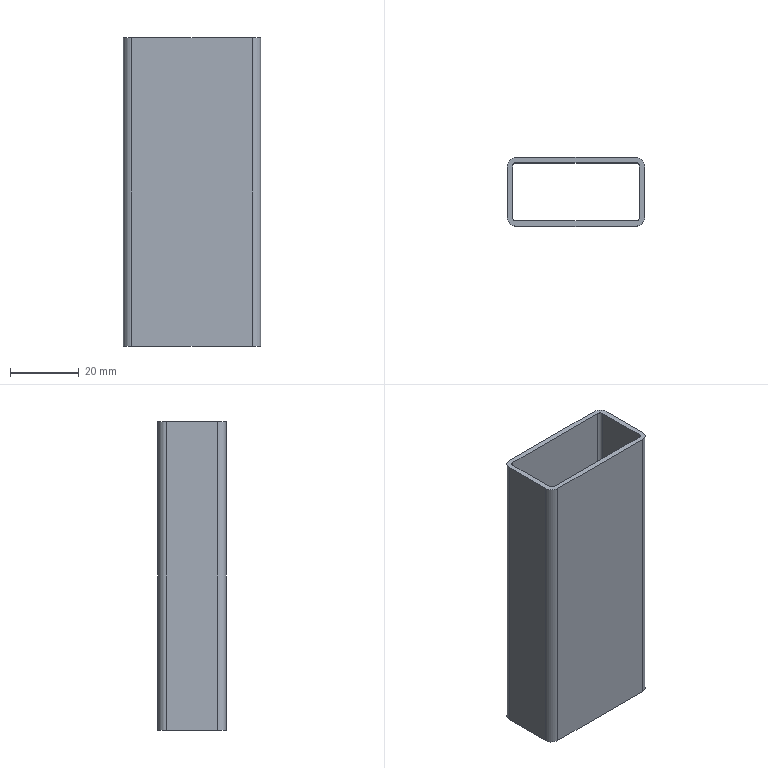Part | STEP file | 6100517 | 1 solid | 18 faces | box 40 x 20 x 90 mm | volume 14984 mm3 | plane 10 | cylinder 8 | commonest cylinder face diameters 2 x4 5 x4
STEP:
#1=CARTESIAN_POINT('',(0.,0.,0.));
#2=DIRECTION('',(0.,0.,1.));
#3=DIRECTION('',(1.,0.,0.));
#4=AXIS2_PLACEMENT_3D('',#1,#2,#3);
#5=CARTESIAN_POINT('',(-17.5,10.,90.));
#6=VERTEX_POINT('',#5);
#7=CARTESIAN_POINT('',(-20.,7.5,90.));
#8=VERTEX_POINT('',#7);
#9=CARTESIAN_POINT('',(-17.5,7.5,90.));
#10=DIRECTION('',(0.,0.,1.));
#11=DIRECTION('',(1.,0.,0.));
#12=AXIS2_PLACEMENT_3D('',#9,#10,#11);
#13=CIRCLE('',#12,2.5);
#14=CARTESIAN_POINT('',(-17.5,7.5,90.));
#15=DIRECTION('',(0.,0.,1.));
#16=DIRECTION('',(1.,0.,0.));
#17=AXIS2_PLACEMENT_3D('',#14,#15,#16);
#18=PLANE('',#17);
#19=CARTESIAN_POINT('',(0.,0.));
#20=DIRECTION('',(1.,0.));
#21=AXIS2_PLACEMENT_2D('',#19,#20);
#22=CIRCLE('',#21,2.5);
#23=(GEOMETRIC_REPRESENTATION_CONTEXT(2)PARAMETRIC_REPRESENTATION_CONTEXT()REPRESENTATION_CONTEXT('',''));
#24=DEFINITIONAL_REPRESENTATION('',(#22),#23);
#25=PCURVE('',#18,#24);
#26=CARTESIAN_POINT('',(-17.5,7.5,90.));
#27=DIRECTION('',(0.,0.,-1.));
#28=DIRECTION('',(-1.,0.,0.));
#29=AXIS2_PLACEMENT_3D('',#26,#27,#28);
#30=CYLINDRICAL_SURFACE('',#29,2.5);
#31=CARTESIAN_POINT('',(3.142,0.));
#32=DIRECTION('',(-1.,0.));
#33=VECTOR('',#32,1.);
#34=LINE('',#31,#33);
#35=(GEOMETRIC_REPRESENTATION_CONTEXT(2)PARAMETRIC_REPRESENTATION_CONTEXT()REPRESENTATION_CONTEXT('',''));
#36=DEFINITIONAL_REPRESENTATION('',(#34),#35);
#37=PCURVE('',#30,#36);
#38=SURFACE_CURVE('',#13,(#25,#37),.PCURVE_S1.);
#39=EDGE_CURVE('',#6,#8,#38,.T.);
#40=ORIENTED_EDGE('',*,*,#39,.T.);
#41=CARTESIAN_POINT('',(-20.,-7.5,90.));
#42=VERTEX_POINT('',#41);
#43=CARTESIAN_POINT('',(-20.,7.5,90.));
#44=DIRECTION('',(0.,-1.,0.));
#45=VECTOR('',#44,1.);
#46=LINE('',#43,#45);
#47=CARTESIAN_POINT('',(-2.5,0.));
#48=DIRECTION('',(0.,-1.));
#49=VECTOR('',#48,1.);
#50=LINE('',#47,#49);
#51=(GEOMETRIC_REPRESENTATION_CONTEXT(2)PARAMETRIC_REPRESENTATION_CONTEXT()REPRESENTATION_CONTEXT('',''));
#52=DEFINITIONAL_REPRESENTATION('',(#50),#51);
#53=PCURVE('',#18,#52);
#54=CARTESIAN_POINT('',(-20.,7.5,90.));
#55=DIRECTION('',(1.,0.,0.));
#56=DIRECTION('',(0.,1.,0.));
#57=AXIS2_PLACEMENT_3D('',#54,#55,#56);
#58=PLANE('',#57);
#59=CARTESIAN_POINT('',(0.,0.));
#60=DIRECTION('',(-1.,0.));
#61=VECTOR('',#60,1.);
#62=LINE('',#59,#61);
#63=(GEOMETRIC_REPRESENTATION_CONTEXT(2)PARAMETRIC_REPRESENTATION_CONTEXT()REPRESENTATION_CONTEXT('',''));
#64=DEFINITIONAL_REPRESENTATION('',(#62),#63);
#65=PCURVE('',#58,#64);
#66=SURFACE_CURVE('',#46,(#53,#65),.PCURVE_S1.);
#67=EDGE_CURVE('',#8,#42,#66,.T.);
#68=ORIENTED_EDGE('',*,*,#67,.T.);
#69=CARTESIAN_POINT('',(-17.5,-10.,90.));
#70=VERTEX_POINT('',#69);
#71=CARTESIAN_POINT('',(-17.5,-7.5,90.));
#72=DIRECTION('',(0.,0.,1.));
#73=DIRECTION('',(1.,0.,0.));
#74=AXIS2_PLACEMENT_3D('',#71,#72,#73);
#75=CIRCLE('',#74,2.5);
#76=CARTESIAN_POINT('',(0.,-15.));
#77=DIRECTION('',(1.,0.));
#78=AXIS2_PLACEMENT_2D('',#76,#77);
#79=CIRCLE('',#78,2.5);
#80=(GEOMETRIC_REPRESENTATION_CONTEXT(2)PARAMETRIC_REPRESENTATION_CONTEXT()REPRESENTATION_CONTEXT('',''));
#81=DEFINITIONAL_REPRESENTATION('',(#79),#80);
#82=PCURVE('',#18,#81);
#83=CARTESIAN_POINT('',(-17.5,-7.5,90.));
#84=DIRECTION('',(0.,0.,-1.));
#85=DIRECTION('',(-1.,0.,0.));
#86=AXIS2_PLACEMENT_3D('',#83,#84,#85);
#87=CYLINDRICAL_SURFACE('',#86,2.5);
#88=CARTESIAN_POINT('',(9.425,0.));
#89=DIRECTION('',(-1.,0.));
#90=VECTOR('',#89,1.);
#91=LINE('',#88,#90);
#92=(GEOMETRIC_REPRESENTATION_CONTEXT(2)PARAMETRIC_REPRESENTATION_CONTEXT()REPRESENTATION_CONTEXT('',''));
#93=DEFINITIONAL_REPRESENTATION('',(#91),#92);
#94=PCURVE('',#87,#93);
#95=SURFACE_CURVE('',#75,(#82,#94),.PCURVE_S1.);
#96=EDGE_CURVE('',#42,#70,#95,.T.);
#97=ORIENTED_EDGE('',*,*,#96,.T.);
#98=CARTESIAN_POINT('',(17.5,-10.,90.));
#99=VERTEX_POINT('',#98);
#100=CARTESIAN_POINT('',(-17.5,-10.,90.));
#101=DIRECTION('',(1.,0.,0.));
#102=VECTOR('',#101,1.);
#103=LINE('',#100,#102);
#104=CARTESIAN_POINT('',(0.,-17.5));
#105=DIRECTION('',(1.,0.));
#106=VECTOR('',#105,1.);
#107=LINE('',#104,#106);
#108=(GEOMETRIC_REPRESENTATION_CONTEXT(2)PARAMETRIC_REPRESENTATION_CONTEXT()REPRESENTATION_CONTEXT('',''));
#109=DEFINITIONAL_REPRESENTATION('',(#107),#108);
#110=PCURVE('',#18,#109);
#111=CARTESIAN_POINT('',(-17.5,-10.,90.));
#112=DIRECTION('',(0.,1.,0.));
#113=DIRECTION('',(0.,0.,1.));
#114=AXIS2_PLACEMENT_3D('',#111,#112,#113);
#115=PLANE('',#114);
#116=CARTESIAN_POINT('',(0.,0.));
#117=DIRECTION('',(0.,1.));
#118=VECTOR('',#117,1.);
#119=LINE('',#116,#118);
#120=(GEOMETRIC_REPRESENTATION_CONTEXT(2)PARAMETRIC_REPRESENTATION_CONTEXT()REPRESENTATION_CONTEXT('',''));
#121=DEFINITIONAL_REPRESENTATION('',(#119),#120);
#122=PCURVE('',#115,#121);
#123=SURFACE_CURVE('',#103,(#110,#122),.PCURVE_S1.);
#124=EDGE_CURVE('',#70,#99,#123,.T.);
#125=ORIENTED_EDGE('',*,*,#124,.T.);
#126=CARTESIAN_POINT('',(20.,-7.5,90.));
#127=VERTEX_POINT('',#126);
#128=CARTESIAN_POINT('',(17.5,-7.5,90.));
#129=DIRECTION('',(0.,0.,1.));
#130=DIRECTION('',(1.,0.,0.));
#131=AXIS2_PLACEMENT_3D('',#128,#129,#130);
#132=CIRCLE('',#131,2.5);
#133=CARTESIAN_POINT('',(35.,-15.));
#134=DIRECTION('',(1.,0.));
#135=AXIS2_PLACEMENT_2D('',#133,#134);
#136=CIRCLE('',#135,2.5);
#137=(GEOMETRIC_REPRESENTATION_CONTEXT(2)PARAMETRIC_REPRESENTATION_CONTEXT()REPRESENTATION_CONTEXT('',''));
#138=DEFINITIONAL_REPRESENTATION('',(#136),#137);
#139=PCURVE('',#18,#138);
#140=CARTESIAN_POINT('',(17.5,-7.5,90.));
#141=DIRECTION('',(0.,0.,-1.));
#142=DIRECTION('',(-1.,0.,0.));
#143=AXIS2_PLACEMENT_3D('',#140,#141,#142);
#144=CYLINDRICAL_SURFACE('',#143,2.5);
#145=CARTESIAN_POINT('',(9.425,0.));
#146=DIRECTION('',(-1.,0.));
#147=VECTOR('',#146,1.);
#148=LINE('',#145,#147);
#149=(GEOMETRIC_REPRESENTATION_CONTEXT(2)PARAMETRIC_REPRESENTATION_CONTEXT()REPRESENTATION_CONTEXT('',''));
#150=DEFINITIONAL_REPRESENTATION('',(#148),#149);
#151=PCURVE('',#144,#150);
#152=SURFACE_CURVE('',#132,(#139,#151),.PCURVE_S1.);
#153=EDGE_CURVE('',#99,#127,#152,.T.);
#154=ORIENTED_EDGE('',*,*,#153,.T.);
#155=CARTESIAN_POINT('',(20.,7.5,90.));
#156=VERTEX_POINT('',#155);
#157=CARTESIAN_POINT('',(20.,7.5,90.));
#158=DIRECTION('',(0.,1.,0.));
#159=VECTOR('',#158,1.);
#160=LINE('',#157,#159);
#161=CARTESIAN_POINT('',(37.5,0.));
#162=DIRECTION('',(0.,1.));
#163=VECTOR('',#162,1.);
#164=LINE('',#161,#163);
#165=(GEOMETRIC_REPRESENTATION_CONTEXT(2)PARAMETRIC_REPRESENTATION_CONTEXT()REPRESENTATION_CONTEXT('',''));
#166=DEFINITIONAL_REPRESENTATION('',(#164),#165);
#167=PCURVE('',#18,#166);
#168=CARTESIAN_POINT('',(20.,7.5,90.));
#169=DIRECTION('',(-1.,0.,0.));
#170=DIRECTION('',(0.,-1.,0.));
#171=AXIS2_PLACEMENT_3D('',#168,#169,#170);
#172=PLANE('',#171);
#173=CARTESIAN_POINT('',(0.,0.));
#174=DIRECTION('',(-1.,0.));
#175=VECTOR('',#174,1.);
#176=LINE('',#173,#175);
#177=(GEOMETRIC_REPRESENTATION_CONTEXT(2)PARAMETRIC_REPRESENTATION_CONTEXT()REPRESENTATION_CONTEXT('',''));
#178=DEFINITIONAL_REPRESENTATION('',(#176),#177);
#179=PCURVE('',#172,#178);
#180=SURFACE_CURVE('',#160,(#167,#179),.PCURVE_S1.);
#181=EDGE_CURVE('',#127,#156,#180,.T.);
#182=ORIENTED_EDGE('',*,*,#181,.T.);
#183=CARTESIAN_POINT('',(17.5,10.,90.));
#184=VERTEX_POINT('',#183);
#185=CARTESIAN_POINT('',(17.5,7.5,90.));
#186=DIRECTION('',(0.,0.,1.));
#187=DIRECTION('',(-1.,0.,0.));
#188=AXIS2_PLACEMENT_3D('',#185,#186,#187);
#189=CIRCLE('',#188,2.5);
#190=CARTESIAN_POINT('',(35.,0.));
#191=DIRECTION('',(-1.,0.));
#192=AXIS2_PLACEMENT_2D('',#190,#191);
#193=CIRCLE('',#192,2.5);
#194=(GEOMETRIC_REPRESENTATION_CONTEXT(2)PARAMETRIC_REPRESENTATION_CONTEXT()REPRESENTATION_CONTEXT('',''));
#195=DEFINITIONAL_REPRESENTATION('',(#193),#194);
#196=PCURVE('',#18,#195);
#197=CARTESIAN_POINT('',(17.5,7.5,90.));
#198=DIRECTION('',(0.,0.,-1.));
#199=DIRECTION('',(-1.,0.,0.));
#200=AXIS2_PLACEMENT_3D('',#197,#198,#199);
#201=CYLINDRICAL_SURFACE('',#200,2.5);
#202=CARTESIAN_POINT('',(6.283,0.));
#203=DIRECTION('',(-1.,0.));
#204=VECTOR('',#203,1.);
#205=LINE('',#202,#204);
#206=(GEOMETRIC_REPRESENTATION_CONTEXT(2)PARAMETRIC_REPRESENTATION_CONTEXT()REPRESENTATION_CONTEXT('',''));
#207=DEFINITIONAL_REPRESENTATION('',(#205),#206);
#208=PCURVE('',#201,#207);
#209=SURFACE_CURVE('',#189,(#196,#208),.PCURVE_S1.);
#210=EDGE_CURVE('',#156,#184,#209,.T.);
#211=ORIENTED_EDGE('',*,*,#210,.T.);
#212=CARTESIAN_POINT('',(-17.5,10.,90.));
#213=DIRECTION('',(-1.,0.,0.));
#214=VECTOR('',#213,1.);
#215=LINE('',#212,#214);
#216=CARTESIAN_POINT('',(0.,2.5));
#217=DIRECTION('',(-1.,0.));
#218=VECTOR('',#217,1.);
#219=LINE('',#216,#218);
#220=(GEOMETRIC_REPRESENTATION_CONTEXT(2)PARAMETRIC_REPRESENTATION_CONTEXT()REPRESENTATION_CONTEXT('',''));
#221=DEFINITIONAL_REPRESENTATION('',(#219),#220);
#222=PCURVE('',#18,#221);
#223=CARTESIAN_POINT('',(-17.5,10.,90.));
#224=DIRECTION('',(0.,-1.,0.));
#225=DIRECTION('',(0.,0.,-1.));
#226=AXIS2_PLACEMENT_3D('',#223,#224,#225);
#227=PLANE('',#226);
#228=CARTESIAN_POINT('',(0.,0.));
#229=DIRECTION('',(0.,-1.));
#230=VECTOR('',#229,1.);
#231=LINE('',#228,#230);
#232=(GEOMETRIC_REPRESENTATION_CONTEXT(2)PARAMETRIC_REPRESENTATION_CONTEXT()REPRESENTATION_CONTEXT('',''));
#233=DEFINITIONAL_REPRESENTATION('',(#231),#232);
#234=PCURVE('',#227,#233);
#235=SURFACE_CURVE('',#215,(#222,#234),.PCURVE_S1.);
#236=EDGE_CURVE('',#184,#6,#235,.T.);
#237=ORIENTED_EDGE('',*,*,#236,.T.);
#238=EDGE_LOOP('',(#40,#68,#97,#125,#154,#182,#211,#237));
#239=FACE_BOUND('',#238,.T.);
#240=CARTESIAN_POINT('',(-18.5,7.5,90.));
#241=VERTEX_POINT('',#240);
#242=CARTESIAN_POINT('',(-18.5,-7.5,90.));
#243=VERTEX_POINT('',#242);
#244=CARTESIAN_POINT('',(-18.5,7.5,90.));
#245=DIRECTION('',(0.,-1.,0.));
#246=VECTOR('',#245,1.);
#247=LINE('',#244,#246);
#248=CARTESIAN_POINT('',(-1.,0.));
#249=DIRECTION('',(0.,-1.));
#250=VECTOR('',#249,1.);
#251=LINE('',#248,#250);
#252=(GEOMETRIC_REPRESENTATION_CONTEXT(2)PARAMETRIC_REPRESENTATION_CONTEXT()REPRESENTATION_CONTEXT('',''));
#253=DEFINITIONAL_REPRESENTATION('',(#251),#252);
#254=PCURVE('',#18,#253);
#255=CARTESIAN_POINT('',(-18.5,7.5,90.));
#256=DIRECTION('',(1.,0.,0.));
#257=DIRECTION('',(0.,0.,-1.));
#258=AXIS2_PLACEMENT_3D('',#255,#256,#257);
#259=PLANE('',#258);
#260=CARTESIAN_POINT('',(0.,0.));
#261=DIRECTION('',(0.,-1.));
#262=VECTOR('',#261,1.);
#263=LINE('',#260,#262);
#264=(GEOMETRIC_REPRESENTATION_CONTEXT(2)PARAMETRIC_REPRESENTATION_CONTEXT()REPRESENTATION_CONTEXT('',''));
#265=DEFINITIONAL_REPRESENTATION('',(#263),#264);
#266=PCURVE('',#259,#265);
#267=SURFACE_CURVE('',#247,(#254,#266),.PCURVE_S1.);
#268=EDGE_CURVE('',#241,#243,#267,.T.);
#269=ORIENTED_EDGE('',*,*,#268,.F.);
#270=CARTESIAN_POINT('',(-17.5,8.5,90.));
#271=VERTEX_POINT('',#270);
#272=CARTESIAN_POINT('',(-17.5,7.5,90.));
#273=DIRECTION('',(0.,0.,1.));
#274=DIRECTION('',(1.,0.,0.));
#275=AXIS2_PLACEMENT_3D('',#272,#273,#274);
#276=CIRCLE('',#275,1.);
#277=CARTESIAN_POINT('',(0.,0.));
#278=DIRECTION('',(1.,0.));
#279=AXIS2_PLACEMENT_2D('',#277,#278);
#280=CIRCLE('',#279,1.);
#281=(GEOMETRIC_REPRESENTATION_CONTEXT(2)PARAMETRIC_REPRESENTATION_CONTEXT()REPRESENTATION_CONTEXT('',''));
#282=DEFINITIONAL_REPRESENTATION('',(#280),#281);
#283=PCURVE('',#18,#282);
#284=CARTESIAN_POINT('',(-17.5,7.5,90.));
#285=DIRECTION('',(0.,0.,-1.));
#286=DIRECTION('',(-1.,0.,0.));
#287=AXIS2_PLACEMENT_3D('',#284,#285,#286);
#288=CYLINDRICAL_SURFACE('',#287,1.);
#289=CARTESIAN_POINT('',(3.142,0.));
#290=DIRECTION('',(-1.,0.));
#291=VECTOR('',#290,1.);
#292=LINE('',#289,#291);
#293=(GEOMETRIC_REPRESENTATION_CONTEXT(2)PARAMETRIC_REPRESENTATION_CONTEXT()REPRESENTATION_CONTEXT('',''));
#294=DEFINITIONAL_REPRESENTATION('',(#292),#293);
#295=PCURVE('',#288,#294);
#296=SURFACE_CURVE('',#276,(#283,#295),.PCURVE_S1.);
#297=EDGE_CURVE('',#271,#241,#296,.T.);
#298=ORIENTED_EDGE('',*,*,#297,.F.);
#299=CARTESIAN_POINT('',(17.5,8.5,90.));
#300=VERTEX_POINT('',#299);
#301=CARTESIAN_POINT('',(-17.5,8.5,90.));
#302=DIRECTION('',(-1.,0.,0.));
#303=VECTOR('',#302,1.);
#304=LINE('',#301,#303);
#305=CARTESIAN_POINT('',(0.,1.));
#306=DIRECTION('',(-1.,0.));
#307=VECTOR('',#306,1.);
#308=LINE('',#305,#307);
#309=(GEOMETRIC_REPRESENTATION_CONTEXT(2)PARAMETRIC_REPRESENTATION_CONTEXT()REPRESENTATION_CONTEXT('',''));
#310=DEFINITIONAL_REPRESENTATION('',(#308),#309);
#311=PCURVE('',#18,#310);
#312=CARTESIAN_POINT('',(-17.5,8.5,90.));
#313=DIRECTION('',(0.,-1.,0.));
#314=DIRECTION('',(0.,0.,-1.));
#315=AXIS2_PLACEMENT_3D('',#312,#313,#314);
#316=PLANE('',#315);
#317=CARTESIAN_POINT('',(0.,0.));
#318=DIRECTION('',(0.,-1.));
#319=VECTOR('',#318,1.);
#320=LINE('',#317,#319);
#321=(GEOMETRIC_REPRESENTATION_CONTEXT(2)PARAMETRIC_REPRESENTATION_CONTEXT()REPRESENTATION_CONTEXT('',''));
#322=DEFINITIONAL_REPRESENTATION('',(#320),#321);
#323=PCURVE('',#316,#322);
#324=SURFACE_CURVE('',#304,(#311,#323),.PCURVE_S1.);
#325=EDGE_CURVE('',#300,#271,#324,.T.);
#326=ORIENTED_EDGE('',*,*,#325,.F.);
#327=CARTESIAN_POINT('',(18.5,7.5,90.));
#328=VERTEX_POINT('',#327);
#329=CARTESIAN_POINT('',(17.5,7.5,90.));
#330=DIRECTION('',(0.,0.,1.));
#331=DIRECTION('',(-1.,0.,0.));
#332=AXIS2_PLACEMENT_3D('',#329,#330,#331);
#333=CIRCLE('',#332,1.);
#334=CARTESIAN_POINT('',(35.,0.));
#335=DIRECTION('',(-1.,0.));
#336=AXIS2_PLACEMENT_2D('',#334,#335);
#337=CIRCLE('',#336,1.);
#338=(GEOMETRIC_REPRESENTATION_CONTEXT(2)PARAMETRIC_REPRESENTATION_CONTEXT()REPRESENTATION_CONTEXT('',''));
#339=DEFINITIONAL_REPRESENTATION('',(#337),#338);
#340=PCURVE('',#18,#339);
#341=CARTESIAN_POINT('',(17.5,7.5,90.));
#342=DIRECTION('',(0.,0.,-1.));
#343=DIRECTION('',(-1.,0.,0.));
#344=AXIS2_PLACEMENT_3D('',#341,#342,#343);
#345=CYLINDRICAL_SURFACE('',#344,1.);
#346=CARTESIAN_POINT('',(6.283,0.));
#347=DIRECTION('',(-1.,0.));
#348=VECTOR('',#347,1.);
#349=LINE('',#346,#348);
#350=(GEOMETRIC_REPRESENTATION_CONTEXT(2)PARAMETRIC_REPRESENTATION_CONTEXT()REPRESENTATION_CONTEXT('',''));
#351=DEFINITIONAL_REPRESENTATION('',(#349),#350);
#352=PCURVE('',#345,#351);
#353=SURFACE_CURVE('',#333,(#340,#352),.PCURVE_S1.);
#354=EDGE_CURVE('',#328,#300,#353,.T.);
#355=ORIENTED_EDGE('',*,*,#354,.F.);
#356=CARTESIAN_POINT('',(18.5,-7.5,90.));
#357=VERTEX_POINT('',#356);
#358=CARTESIAN_POINT('',(18.5,7.5,90.));
#359=DIRECTION('',(0.,1.,0.));
#360=VECTOR('',#359,1.);
#361=LINE('',#358,#360);
#362=CARTESIAN_POINT('',(36.,0.));
#363=DIRECTION('',(0.,1.));
#364=VECTOR('',#363,1.);
#365=LINE('',#362,#364);
#366=(GEOMETRIC_REPRESENTATION_CONTEXT(2)PARAMETRIC_REPRESENTATION_CONTEXT()REPRESENTATION_CONTEXT('',''));
#367=DEFINITIONAL_REPRESENTATION('',(#365),#366);
#368=PCURVE('',#18,#367);
#369=CARTESIAN_POINT('',(18.5,7.5,90.));
#370=DIRECTION('',(-1.,0.,0.));
#371=DIRECTION('',(0.,-1.,0.));
#372=AXIS2_PLACEMENT_3D('',#369,#370,#371);
#373=PLANE('',#372);
#374=CARTESIAN_POINT('',(0.,0.));
#375=DIRECTION('',(-1.,0.));
#376=VECTOR('',#375,1.);
#377=LINE('',#374,#376);
#378=(GEOMETRIC_REPRESENTATION_CONTEXT(2)PARAMETRIC_REPRESENTATION_CONTEXT()REPRESENTATION_CONTEXT('',''));
#379=DEFINITIONAL_REPRESENTATION('',(#377),#378);
#380=PCURVE('',#373,#379);
#381=SURFACE_CURVE('',#361,(#368,#380),.PCURVE_S1.);
#382=EDGE_CURVE('',#357,#328,#381,.T.);
#383=ORIENTED_EDGE('',*,*,#382,.F.);
#384=CARTESIAN_POINT('',(17.5,-8.5,90.));
#385=VERTEX_POINT('',#384);
#386=CARTESIAN_POINT('',(17.5,-7.5,90.));
#387=DIRECTION('',(0.,0.,1.));
#388=DIRECTION('',(1.,0.,0.));
#389=AXIS2_PLACEMENT_3D('',#386,#387,#388);
#390=CIRCLE('',#389,1.);
#391=CARTESIAN_POINT('',(35.,-15.));
#392=DIRECTION('',(1.,0.));
#393=AXIS2_PLACEMENT_2D('',#391,#392);
#394=CIRCLE('',#393,1.);
#395=(GEOMETRIC_REPRESENTATION_CONTEXT(2)PARAMETRIC_REPRESENTATION_CONTEXT()REPRESENTATION_CONTEXT('',''));
#396=DEFINITIONAL_REPRESENTATION('',(#394),#395);
#397=PCURVE('',#18,#396);
#398=CARTESIAN_POINT('',(17.5,-7.5,90.));
#399=DIRECTION('',(0.,0.,-1.));
#400=DIRECTION('',(-1.,0.,0.));
#401=AXIS2_PLACEMENT_3D('',#398,#399,#400);
#402=CYLINDRICAL_SURFACE('',#401,1.);
#403=CARTESIAN_POINT('',(9.425,0.));
#404=DIRECTION('',(-1.,0.));
#405=VECTOR('',#404,1.);
#406=LINE('',#403,#405);
#407=(GEOMETRIC_REPRESENTATION_CONTEXT(2)PARAMETRIC_REPRESENTATION_CONTEXT()REPRESENTATION_CONTEXT('',''));
#408=DEFINITIONAL_REPRESENTATION('',(#406),#407);
#409=PCURVE('',#402,#408);
#410=SURFACE_CURVE('',#390,(#397,#409),.PCURVE_S1.);
#411=EDGE_CURVE('',#385,#357,#410,.T.);
#412=ORIENTED_EDGE('',*,*,#411,.F.);
#413=CARTESIAN_POINT('',(-17.5,-8.5,90.));
#414=VERTEX_POINT('',#413);
#415=CARTESIAN_POINT('',(-17.5,-8.5,90.));
#416=DIRECTION('',(1.,0.,0.));
#417=VECTOR('',#416,1.);
#418=LINE('',#415,#417);
#419=CARTESIAN_POINT('',(0.,-16.));
#420=DIRECTION('',(1.,0.));
#421=VECTOR('',#420,1.);
#422=LINE('',#419,#421);
#423=(GEOMETRIC_REPRESENTATION_CONTEXT(2)PARAMETRIC_REPRESENTATION_CONTEXT()REPRESENTATION_CONTEXT('',''));
#424=DEFINITIONAL_REPRESENTATION('',(#422),#423);
#425=PCURVE('',#18,#424);
#426=CARTESIAN_POINT('',(-17.5,-8.5,90.));
#427=DIRECTION('',(0.,1.,0.));
#428=DIRECTION('',(0.,0.,1.));
#429=AXIS2_PLACEMENT_3D('',#426,#427,#428);
#430=PLANE('',#429);
#431=CARTESIAN_POINT('',(0.,0.));
#432=DIRECTION('',(0.,1.));
#433=VECTOR('',#432,1.);
#434=LINE('',#431,#433);
#435=(GEOMETRIC_REPRESENTATION_CONTEXT(2)PARAMETRIC_REPRESENTATION_CONTEXT()REPRESENTATION_CONTEXT('',''));
#436=DEFINITIONAL_REPRESENTATION('',(#434),#435);
#437=PCURVE('',#430,#436);
#438=SURFACE_CURVE('',#418,(#425,#437),.PCURVE_S1.);
#439=EDGE_CURVE('',#414,#385,#438,.T.);
#440=ORIENTED_EDGE('',*,*,#439,.F.);
#441=CARTESIAN_POINT('',(-17.5,-7.5,90.));
#442=DIRECTION('',(0.,0.,1.));
#443=DIRECTION('',(1.,0.,0.));
#444=AXIS2_PLACEMENT_3D('',#441,#442,#443);
#445=CIRCLE('',#444,1.);
#446=CARTESIAN_POINT('',(0.,-15.));
#447=DIRECTION('',(1.,0.));
#448=AXIS2_PLACEMENT_2D('',#446,#447);
#449=CIRCLE('',#448,1.);
#450=(GEOMETRIC_REPRESENTATION_CONTEXT(2)PARAMETRIC_REPRESENTATION_CONTEXT()REPRESENTATION_CONTEXT('',''));
#451=DEFINITIONAL_REPRESENTATION('',(#449),#450);
#452=PCURVE('',#18,#451);
#453=CARTESIAN_POINT('',(-17.5,-7.5,90.));
#454=DIRECTION('',(0.,0.,-1.));
#455=DIRECTION('',(-1.,0.,0.));
#456=AXIS2_PLACEMENT_3D('',#453,#454,#455);
#457=CYLINDRICAL_SURFACE('',#456,1.);
#458=CARTESIAN_POINT('',(9.425,0.));
#459=DIRECTION('',(-1.,0.));
#460=VECTOR('',#459,1.);
#461=LINE('',#458,#460);
#462=(GEOMETRIC_REPRESENTATION_CONTEXT(2)PARAMETRIC_REPRESENTATION_CONTEXT()REPRESENTATION_CONTEXT('',''));
#463=DEFINITIONAL_REPRESENTATION('',(#461),#462);
#464=PCURVE('',#457,#463);
#465=SURFACE_CURVE('',#445,(#452,#464),.PCURVE_S1.);
#466=EDGE_CURVE('',#243,#414,#465,.T.);
#467=ORIENTED_EDGE('',*,*,#466,.F.);
#468=EDGE_LOOP('',(#269,#298,#326,#355,#383,#412,#440,#467));
#469=FACE_BOUND('',#468,.T.);
#470=ADVANCED_FACE('',(#239,#469),#18,.T.);
#471=CARTESIAN_POINT('',(-17.5,10.,0.));
#472=VERTEX_POINT('',#471);
#473=CARTESIAN_POINT('',(-20.,7.5,0.));
#474=VERTEX_POINT('',#473);
#475=CARTESIAN_POINT('',(-17.5,7.5,0.));
#476=DIRECTION('',(0.,0.,1.));
#477=DIRECTION('',(1.,0.,0.));
#478=AXIS2_PLACEMENT_3D('',#475,#476,#477);
#479=CIRCLE('',#478,2.5);
#480=CARTESIAN_POINT('',(-17.5,7.5,0.));
#481=DIRECTION('',(0.,0.,1.));
#482=DIRECTION('',(1.,0.,0.));
#483=AXIS2_PLACEMENT_3D('',#480,#481,#482);
#484=PLANE('',#483);
#485=CARTESIAN_POINT('',(0.,0.));
#486=DIRECTION('',(1.,0.));
#487=AXIS2_PLACEMENT_2D('',#485,#486);
#488=CIRCLE('',#487,2.5);
#489=(GEOMETRIC_REPRESENTATION_CONTEXT(2)PARAMETRIC_REPRESENTATION_CONTEXT()REPRESENTATION_CONTEXT('',''));
#490=DEFINITIONAL_REPRESENTATION('',(#488),#489);
#491=PCURVE('',#484,#490);
#492=CARTESIAN_POINT('',(3.142,90.));
#493=DIRECTION('',(-1.,0.));
#494=VECTOR('',#493,1.);
#495=LINE('',#492,#494);
#496=(GEOMETRIC_REPRESENTATION_CONTEXT(2)PARAMETRIC_REPRESENTATION_CONTEXT()REPRESENTATION_CONTEXT('',''));
#497=DEFINITIONAL_REPRESENTATION('',(#495),#496);
#498=PCURVE('',#30,#497);
#499=SURFACE_CURVE('',#479,(#491,#498),.PCURVE_S1.);
#500=EDGE_CURVE('',#472,#474,#499,.T.);
#501=ORIENTED_EDGE('',*,*,#500,.F.);
#502=CARTESIAN_POINT('',(17.5,10.,0.));
#503=VERTEX_POINT('',#502);
#504=CARTESIAN_POINT('',(-17.5,10.,0.));
#505=DIRECTION('',(-1.,0.,0.));
#506=VECTOR('',#505,1.);
#507=LINE('',#504,#506);
#508=CARTESIAN_POINT('',(0.,2.5));
#509=DIRECTION('',(-1.,0.));
#510=VECTOR('',#509,1.);
#511=LINE('',#508,#510);
#512=(GEOMETRIC_REPRESENTATION_CONTEXT(2)PARAMETRIC_REPRESENTATION_CONTEXT()REPRESENTATION_CONTEXT('',''));
#513=DEFINITIONAL_REPRESENTATION('',(#511),#512);
#514=PCURVE('',#484,#513);
#515=CARTESIAN_POINT('',(90.,0.));
#516=DIRECTION('',(0.,-1.));
#517=VECTOR('',#516,1.);
#518=LINE('',#515,#517);
#519=(GEOMETRIC_REPRESENTATION_CONTEXT(2)PARAMETRIC_REPRESENTATION_CONTEXT()REPRESENTATION_CONTEXT('',''));
#520=DEFINITIONAL_REPRESENTATION('',(#518),#519);
#521=PCURVE('',#227,#520);
#522=SURFACE_CURVE('',#507,(#514,#521),.PCURVE_S1.);
#523=EDGE_CURVE('',#503,#472,#522,.T.);
#524=ORIENTED_EDGE('',*,*,#523,.F.);
#525=CARTESIAN_POINT('',(20.,7.5,0.));
#526=VERTEX_POINT('',#525);
#527=CARTESIAN_POINT('',(17.5,7.5,0.));
#528=DIRECTION('',(0.,0.,1.));
#529=DIRECTION('',(-1.,0.,0.));
#530=AXIS2_PLACEMENT_3D('',#527,#528,#529);
#531=CIRCLE('',#530,2.5);
#532=CARTESIAN_POINT('',(35.,0.));
#533=DIRECTION('',(-1.,0.));
#534=AXIS2_PLACEMENT_2D('',#532,#533);
#535=CIRCLE('',#534,2.5);
#536=(GEOMETRIC_REPRESENTATION_CONTEXT(2)PARAMETRIC_REPRESENTATION_CONTEXT()REPRESENTATION_CONTEXT('',''));
#537=DEFINITIONAL_REPRESENTATION('',(#535),#536);
#538=PCURVE('',#484,#537);
#539=CARTESIAN_POINT('',(6.283,90.));
#540=DIRECTION('',(-1.,0.));
#541=VECTOR('',#540,1.);
#542=LINE('',#539,#541);
#543=(GEOMETRIC_REPRESENTATION_CONTEXT(2)PARAMETRIC_REPRESENTATION_CONTEXT()REPRESENTATION_CONTEXT('',''));
#544=DEFINITIONAL_REPRESENTATION('',(#542),#543);
#545=PCURVE('',#201,#544);
#546=SURFACE_CURVE('',#531,(#538,#545),.PCURVE_S1.);
#547=EDGE_CURVE('',#526,#503,#546,.T.);
#548=ORIENTED_EDGE('',*,*,#547,.F.);
#549=CARTESIAN_POINT('',(20.,-7.5,0.));
#550=VERTEX_POINT('',#549);
#551=CARTESIAN_POINT('',(20.,7.5,0.));
#552=DIRECTION('',(0.,1.,0.));
#553=VECTOR('',#552,1.);
#554=LINE('',#551,#553);
#555=CARTESIAN_POINT('',(37.5,0.));
#556=DIRECTION('',(0.,1.));
#557=VECTOR('',#556,1.);
#558=LINE('',#555,#557);
#559=(GEOMETRIC_REPRESENTATION_CONTEXT(2)PARAMETRIC_REPRESENTATION_CONTEXT()REPRESENTATION_CONTEXT('',''));
#560=DEFINITIONAL_REPRESENTATION('',(#558),#559);
#561=PCURVE('',#484,#560);
#562=CARTESIAN_POINT('',(0.,-90.));
#563=DIRECTION('',(-1.,0.));
#564=VECTOR('',#563,1.);
#565=LINE('',#562,#564);
#566=(GEOMETRIC_REPRESENTATION_CONTEXT(2)PARAMETRIC_REPRESENTATION_CONTEXT()REPRESENTATION_CONTEXT('',''));
#567=DEFINITIONAL_REPRESENTATION('',(#565),#566);
#568=PCURVE('',#172,#567);
#569=SURFACE_CURVE('',#554,(#561,#568),.PCURVE_S1.);
#570=EDGE_CURVE('',#550,#526,#569,.T.);
#571=ORIENTED_EDGE('',*,*,#570,.F.);
#572=CARTESIAN_POINT('',(17.5,-10.,0.));
#573=VERTEX_POINT('',#572);
#574=CARTESIAN_POINT('',(17.5,-7.5,0.));
#575=DIRECTION('',(0.,0.,1.));
#576=DIRECTION('',(1.,0.,0.));
#577=AXIS2_PLACEMENT_3D('',#574,#575,#576);
#578=CIRCLE('',#577,2.5);
#579=CARTESIAN_POINT('',(35.,-15.));
#580=DIRECTION('',(1.,0.));
#581=AXIS2_PLACEMENT_2D('',#579,#580);
#582=CIRCLE('',#581,2.5);
#583=(GEOMETRIC_REPRESENTATION_CONTEXT(2)PARAMETRIC_REPRESENTATION_CONTEXT()REPRESENTATION_CONTEXT('',''));
#584=DEFINITIONAL_REPRESENTATION('',(#582),#583);
#585=PCURVE('',#484,#584);
#586=CARTESIAN_POINT('',(9.425,90.));
#587=DIRECTION('',(-1.,0.));
#588=VECTOR('',#587,1.);
#589=LINE('',#586,#588);
#590=(GEOMETRIC_REPRESENTATION_CONTEXT(2)PARAMETRIC_REPRESENTATION_CONTEXT()REPRESENTATION_CONTEXT('',''));
#591=DEFINITIONAL_REPRESENTATION('',(#589),#590);
#592=PCURVE('',#144,#591);
#593=SURFACE_CURVE('',#578,(#585,#592),.PCURVE_S1.);
#594=EDGE_CURVE('',#573,#550,#593,.T.);
#595=ORIENTED_EDGE('',*,*,#594,.F.);
#596=CARTESIAN_POINT('',(-17.5,-10.,0.));
#597=VERTEX_POINT('',#596);
#598=CARTESIAN_POINT('',(-17.5,-10.,0.));
#599=DIRECTION('',(1.,0.,0.));
#600=VECTOR('',#599,1.);
#601=LINE('',#598,#600);
#602=CARTESIAN_POINT('',(0.,-17.5));
#603=DIRECTION('',(1.,0.));
#604=VECTOR('',#603,1.);
#605=LINE('',#602,#604);
#606=(GEOMETRIC_REPRESENTATION_CONTEXT(2)PARAMETRIC_REPRESENTATION_CONTEXT()REPRESENTATION_CONTEXT('',''));
#607=DEFINITIONAL_REPRESENTATION('',(#605),#606);
#608=PCURVE('',#484,#607);
#609=CARTESIAN_POINT('',(-90.,0.));
#610=DIRECTION('',(0.,1.));
#611=VECTOR('',#610,1.);
#612=LINE('',#609,#611);
#613=(GEOMETRIC_REPRESENTATION_CONTEXT(2)PARAMETRIC_REPRESENTATION_CONTEXT()REPRESENTATION_CONTEXT('',''));
#614=DEFINITIONAL_REPRESENTATION('',(#612),#613);
#615=PCURVE('',#115,#614);
#616=SURFACE_CURVE('',#601,(#608,#615),.PCURVE_S1.);
#617=EDGE_CURVE('',#597,#573,#616,.T.);
#618=ORIENTED_EDGE('',*,*,#617,.F.);
#619=CARTESIAN_POINT('',(-20.,-7.5,0.));
#620=VERTEX_POINT('',#619);
#621=CARTESIAN_POINT('',(-17.5,-7.5,0.));
#622=DIRECTION('',(0.,0.,1.));
#623=DIRECTION('',(1.,0.,0.));
#624=AXIS2_PLACEMENT_3D('',#621,#622,#623);
#625=CIRCLE('',#624,2.5);
#626=CARTESIAN_POINT('',(0.,-15.));
#627=DIRECTION('',(1.,0.));
#628=AXIS2_PLACEMENT_2D('',#626,#627);
#629=CIRCLE('',#628,2.5);
#630=(GEOMETRIC_REPRESENTATION_CONTEXT(2)PARAMETRIC_REPRESENTATION_CONTEXT()REPRESENTATION_CONTEXT('',''));
#631=DEFINITIONAL_REPRESENTATION('',(#629),#630);
#632=PCURVE('',#484,#631);
#633=CARTESIAN_POINT('',(9.425,90.));
#634=DIRECTION('',(-1.,0.));
#635=VECTOR('',#634,1.);
#636=LINE('',#633,#635);
#637=(GEOMETRIC_REPRESENTATION_CONTEXT(2)PARAMETRIC_REPRESENTATION_CONTEXT()REPRESENTATION_CONTEXT('',''));
#638=DEFINITIONAL_REPRESENTATION('',(#636),#637);
#639=PCURVE('',#87,#638);
#640=SURFACE_CURVE('',#625,(#632,#639),.PCURVE_S1.);
#641=EDGE_CURVE('',#620,#597,#640,.T.);
#642=ORIENTED_EDGE('',*,*,#641,.F.);
#643=CARTESIAN_POINT('',(-20.,7.5,0.));
#644=DIRECTION('',(0.,-1.,0.));
#645=VECTOR('',#644,1.);
#646=LINE('',#643,#645);
#647=CARTESIAN_POINT('',(-2.5,0.));
#648=DIRECTION('',(0.,-1.));
#649=VECTOR('',#648,1.);
#650=LINE('',#647,#649);
#651=(GEOMETRIC_REPRESENTATION_CONTEXT(2)PARAMETRIC_REPRESENTATION_CONTEXT()REPRESENTATION_CONTEXT('',''));
#652=DEFINITIONAL_REPRESENTATION('',(#650),#651);
#653=PCURVE('',#484,#652);
#654=CARTESIAN_POINT('',(0.,-90.));
#655=DIRECTION('',(-1.,0.));
#656=VECTOR('',#655,1.);
#657=LINE('',#654,#656);
#658=(GEOMETRIC_REPRESENTATION_CONTEXT(2)PARAMETRIC_REPRESENTATION_CONTEXT()REPRESENTATION_CONTEXT('',''));
#659=DEFINITIONAL_REPRESENTATION('',(#657),#658);
#660=PCURVE('',#58,#659);
#661=SURFACE_CURVE('',#646,(#653,#660),.PCURVE_S1.);
#662=EDGE_CURVE('',#474,#620,#661,.T.);
#663=ORIENTED_EDGE('',*,*,#662,.F.);
#664=EDGE_LOOP('',(#501,#524,#548,#571,#595,#618,#642,#663));
#665=FACE_BOUND('',#664,.T.);
#666=CARTESIAN_POINT('',(-17.5,8.5,0.));
#667=VERTEX_POINT('',#666);
#668=CARTESIAN_POINT('',(-18.5,7.5,0.));
#669=VERTEX_POINT('',#668);
#670=CARTESIAN_POINT('',(-17.5,7.5,0.));
#671=DIRECTION('',(0.,0.,1.));
#672=DIRECTION('',(1.,0.,0.));
#673=AXIS2_PLACEMENT_3D('',#670,#671,#672);
#674=CIRCLE('',#673,1.);
#675=CARTESIAN_POINT('',(0.,0.));
#676=DIRECTION('',(1.,0.));
#677=AXIS2_PLACEMENT_2D('',#675,#676);
#678=CIRCLE('',#677,1.);
#679=(GEOMETRIC_REPRESENTATION_CONTEXT(2)PARAMETRIC_REPRESENTATION_CONTEXT()REPRESENTATION_CONTEXT('',''));
#680=DEFINITIONAL_REPRESENTATION('',(#678),#679);
#681=PCURVE('',#484,#680);
#682=CARTESIAN_POINT('',(3.142,90.));
#683=DIRECTION('',(-1.,0.));
#684=VECTOR('',#683,1.);
#685=LINE('',#682,#684);
#686=(GEOMETRIC_REPRESENTATION_CONTEXT(2)PARAMETRIC_REPRESENTATION_CONTEXT()REPRESENTATION_CONTEXT('',''));
#687=DEFINITIONAL_REPRESENTATION('',(#685),#686);
#688=PCURVE('',#288,#687);
#689=SURFACE_CURVE('',#674,(#681,#688),.PCURVE_S1.);
#690=EDGE_CURVE('',#667,#669,#689,.T.);
#691=ORIENTED_EDGE('',*,*,#690,.T.);
#692=CARTESIAN_POINT('',(-18.5,-7.5,0.));
#693=VERTEX_POINT('',#692);
#694=CARTESIAN_POINT('',(-18.5,7.5,0.));
#695=DIRECTION('',(0.,-1.,0.));
#696=VECTOR('',#695,1.);
#697=LINE('',#694,#696);
#698=CARTESIAN_POINT('',(-1.,0.));
#699=DIRECTION('',(0.,-1.));
#700=VECTOR('',#699,1.);
#701=LINE('',#698,#700);
#702=(GEOMETRIC_REPRESENTATION_CONTEXT(2)PARAMETRIC_REPRESENTATION_CONTEXT()REPRESENTATION_CONTEXT('',''));
#703=DEFINITIONAL_REPRESENTATION('',(#701),#702);
#704=PCURVE('',#484,#703);
#705=CARTESIAN_POINT('',(90.,0.));
#706=DIRECTION('',(0.,-1.));
#707=VECTOR('',#706,1.);
#708=LINE('',#705,#707);
#709=(GEOMETRIC_REPRESENTATION_CONTEXT(2)PARAMETRIC_REPRESENTATION_CONTEXT()REPRESENTATION_CONTEXT('',''));
#710=DEFINITIONAL_REPRESENTATION('',(#708),#709);
#711=PCURVE('',#259,#710);
#712=SURFACE_CURVE('',#697,(#704,#711),.PCURVE_S1.);
#713=EDGE_CURVE('',#669,#693,#712,.T.);
#714=ORIENTED_EDGE('',*,*,#713,.T.);
#715=CARTESIAN_POINT('',(-17.5,-8.5,0.));
#716=VERTEX_POINT('',#715);
#717=CARTESIAN_POINT('',(-17.5,-7.5,0.));
#718=DIRECTION('',(0.,0.,1.));
#719=DIRECTION('',(1.,0.,0.));
#720=AXIS2_PLACEMENT_3D('',#717,#718,#719);
#721=CIRCLE('',#720,1.);
#722=CARTESIAN_POINT('',(0.,-15.));
#723=DIRECTION('',(1.,0.));
#724=AXIS2_PLACEMENT_2D('',#722,#723);
#725=CIRCLE('',#724,1.);
#726=(GEOMETRIC_REPRESENTATION_CONTEXT(2)PARAMETRIC_REPRESENTATION_CONTEXT()REPRESENTATION_CONTEXT('',''));
#727=DEFINITIONAL_REPRESENTATION('',(#725),#726);
#728=PCURVE('',#484,#727);
#729=CARTESIAN_POINT('',(9.425,90.));
#730=DIRECTION('',(-1.,0.));
#731=VECTOR('',#730,1.);
#732=LINE('',#729,#731);
#733=(GEOMETRIC_REPRESENTATION_CONTEXT(2)PARAMETRIC_REPRESENTATION_CONTEXT()REPRESENTATION_CONTEXT('',''));
#734=DEFINITIONAL_REPRESENTATION('',(#732),#733);
#735=PCURVE('',#457,#734);
#736=SURFACE_CURVE('',#721,(#728,#735),.PCURVE_S1.);
#737=EDGE_CURVE('',#693,#716,#736,.T.);
#738=ORIENTED_EDGE('',*,*,#737,.T.);
#739=CARTESIAN_POINT('',(17.5,-8.5,0.));
#740=VERTEX_POINT('',#739);
#741=CARTESIAN_POINT('',(-17.5,-8.5,0.));
#742=DIRECTION('',(1.,0.,0.));
#743=VECTOR('',#742,1.);
#744=LINE('',#741,#743);
#745=CARTESIAN_POINT('',(0.,-16.));
#746=DIRECTION('',(1.,0.));
#747=VECTOR('',#746,1.);
#748=LINE('',#745,#747);
#749=(GEOMETRIC_REPRESENTATION_CONTEXT(2)PARAMETRIC_REPRESENTATION_CONTEXT()REPRESENTATION_CONTEXT('',''));
#750=DEFINITIONAL_REPRESENTATION('',(#748),#749);
#751=PCURVE('',#484,#750);
#752=CARTESIAN_POINT('',(-90.,0.));
#753=DIRECTION('',(0.,1.));
#754=VECTOR('',#753,1.);
#755=LINE('',#752,#754);
#756=(GEOMETRIC_REPRESENTATION_CONTEXT(2)PARAMETRIC_REPRESENTATION_CONTEXT()REPRESENTATION_CONTEXT('',''));
#757=DEFINITIONAL_REPRESENTATION('',(#755),#756);
#758=PCURVE('',#430,#757);
#759=SURFACE_CURVE('',#744,(#751,#758),.PCURVE_S1.);
#760=EDGE_CURVE('',#716,#740,#759,.T.);
#761=ORIENTED_EDGE('',*,*,#760,.T.);
#762=CARTESIAN_POINT('',(18.5,-7.5,0.));
#763=VERTEX_POINT('',#762);
#764=CARTESIAN_POINT('',(17.5,-7.5,0.));
#765=DIRECTION('',(0.,0.,1.));
#766=DIRECTION('',(1.,0.,0.));
#767=AXIS2_PLACEMENT_3D('',#764,#765,#766);
#768=CIRCLE('',#767,1.);
#769=CARTESIAN_POINT('',(35.,-15.));
#770=DIRECTION('',(1.,0.));
#771=AXIS2_PLACEMENT_2D('',#769,#770);
#772=CIRCLE('',#771,1.);
#773=(GEOMETRIC_REPRESENTATION_CONTEXT(2)PARAMETRIC_REPRESENTATION_CONTEXT()REPRESENTATION_CONTEXT('',''));
#774=DEFINITIONAL_REPRESENTATION('',(#772),#773);
#775=PCURVE('',#484,#774);
#776=CARTESIAN_POINT('',(9.425,90.));
#777=DIRECTION('',(-1.,0.));
#778=VECTOR('',#777,1.);
#779=LINE('',#776,#778);
#780=(GEOMETRIC_REPRESENTATION_CONTEXT(2)PARAMETRIC_REPRESENTATION_CONTEXT()REPRESENTATION_CONTEXT('',''));
#781=DEFINITIONAL_REPRESENTATION('',(#779),#780);
#782=PCURVE('',#402,#781);
#783=SURFACE_CURVE('',#768,(#775,#782),.PCURVE_S1.);
#784=EDGE_CURVE('',#740,#763,#783,.T.);
#785=ORIENTED_EDGE('',*,*,#784,.T.);
#786=CARTESIAN_POINT('',(18.5,7.5,0.));
#787=VERTEX_POINT('',#786);
#788=CARTESIAN_POINT('',(18.5,7.5,0.));
#789=DIRECTION('',(0.,1.,0.));
#790=VECTOR('',#789,1.);
#791=LINE('',#788,#790);
#792=CARTESIAN_POINT('',(36.,0.));
#793=DIRECTION('',(0.,1.));
#794=VECTOR('',#793,1.);
#795=LINE('',#792,#794);
#796=(GEOMETRIC_REPRESENTATION_CONTEXT(2)PARAMETRIC_REPRESENTATION_CONTEXT()REPRESENTATION_CONTEXT('',''));
#797=DEFINITIONAL_REPRESENTATION('',(#795),#796);
#798=PCURVE('',#484,#797);
#799=CARTESIAN_POINT('',(0.,-90.));
#800=DIRECTION('',(-1.,0.));
#801=VECTOR('',#800,1.);
#802=LINE('',#799,#801);
#803=(GEOMETRIC_REPRESENTATION_CONTEXT(2)PARAMETRIC_REPRESENTATION_CONTEXT()REPRESENTATION_CONTEXT('',''));
#804=DEFINITIONAL_REPRESENTATION('',(#802),#803);
#805=PCURVE('',#373,#804);
#806=SURFACE_CURVE('',#791,(#798,#805),.PCURVE_S1.);
#807=EDGE_CURVE('',#763,#787,#806,.T.);
#808=ORIENTED_EDGE('',*,*,#807,.T.);
#809=CARTESIAN_POINT('',(17.5,8.5,0.));
#810=VERTEX_POINT('',#809);
#811=CARTESIAN_POINT('',(17.5,7.5,0.));
#812=DIRECTION('',(0.,0.,1.));
#813=DIRECTION('',(-1.,0.,0.));
#814=AXIS2_PLACEMENT_3D('',#811,#812,#813);
#815=CIRCLE('',#814,1.);
#816=CARTESIAN_POINT('',(35.,0.));
#817=DIRECTION('',(-1.,0.));
#818=AXIS2_PLACEMENT_2D('',#816,#817);
#819=CIRCLE('',#818,1.);
#820=(GEOMETRIC_REPRESENTATION_CONTEXT(2)PARAMETRIC_REPRESENTATION_CONTEXT()REPRESENTATION_CONTEXT('',''));
#821=DEFINITIONAL_REPRESENTATION('',(#819),#820);
#822=PCURVE('',#484,#821);
#823=CARTESIAN_POINT('',(6.283,90.));
#824=DIRECTION('',(-1.,0.));
#825=VECTOR('',#824,1.);
#826=LINE('',#823,#825);
#827=(GEOMETRIC_REPRESENTATION_CONTEXT(2)PARAMETRIC_REPRESENTATION_CONTEXT()REPRESENTATION_CONTEXT('',''));
#828=DEFINITIONAL_REPRESENTATION('',(#826),#827);
#829=PCURVE('',#345,#828);
#830=SURFACE_CURVE('',#815,(#822,#829),.PCURVE_S1.);
#831=EDGE_CURVE('',#787,#810,#830,.T.);
#832=ORIENTED_EDGE('',*,*,#831,.T.);
#833=CARTESIAN_POINT('',(-17.5,8.5,0.));
#834=DIRECTION('',(-1.,0.,0.));
#835=VECTOR('',#834,1.);
#836=LINE('',#833,#835);
#837=CARTESIAN_POINT('',(0.,1.));
#838=DIRECTION('',(-1.,0.));
#839=VECTOR('',#838,1.);
#840=LINE('',#837,#839);
#841=(GEOMETRIC_REPRESENTATION_CONTEXT(2)PARAMETRIC_REPRESENTATION_CONTEXT()REPRESENTATION_CONTEXT('',''));
#842=DEFINITIONAL_REPRESENTATION('',(#840),#841);
#843=PCURVE('',#484,#842);
#844=CARTESIAN_POINT('',(90.,0.));
#845=DIRECTION('',(0.,-1.));
#846=VECTOR('',#845,1.);
#847=LINE('',#844,#846);
#848=(GEOMETRIC_REPRESENTATION_CONTEXT(2)PARAMETRIC_REPRESENTATION_CONTEXT()REPRESENTATION_CONTEXT('',''));
#849=DEFINITIONAL_REPRESENTATION('',(#847),#848);
#850=PCURVE('',#316,#849);
#851=SURFACE_CURVE('',#836,(#843,#850),.PCURVE_S1.);
#852=EDGE_CURVE('',#810,#667,#851,.T.);
#853=ORIENTED_EDGE('',*,*,#852,.T.);
#854=EDGE_LOOP('',(#691,#714,#738,#761,#785,#808,#832,#853));
#855=FACE_BOUND('',#854,.T.);
#856=ADVANCED_FACE('',(#665,#855),#484,.F.);
#857=ORIENTED_EDGE('',*,*,#500,.T.);
#858=CARTESIAN_POINT('',(-20.,7.5,90.));
#859=DIRECTION('',(0.,0.,-1.));
#860=VECTOR('',#859,1.);
#861=LINE('',#858,#860);
#862=CARTESIAN_POINT('',(0.,0.));
#863=DIRECTION('',(0.,1.));
#864=VECTOR('',#863,1.);
#865=LINE('',#862,#864);
#866=(GEOMETRIC_REPRESENTATION_CONTEXT(2)PARAMETRIC_REPRESENTATION_CONTEXT()REPRESENTATION_CONTEXT('',''));
#867=DEFINITIONAL_REPRESENTATION('',(#865),#866);
#868=PCURVE('',#30,#867);
#869=CARTESIAN_POINT('',(0.,0.));
#870=DIRECTION('',(0.,-1.));
#871=VECTOR('',#870,1.);
#872=LINE('',#869,#871);
#873=(GEOMETRIC_REPRESENTATION_CONTEXT(2)PARAMETRIC_REPRESENTATION_CONTEXT()REPRESENTATION_CONTEXT('',''));
#874=DEFINITIONAL_REPRESENTATION('',(#872),#873);
#875=PCURVE('',#58,#874);
#876=SURFACE_CURVE('',#861,(#868,#875),.PCURVE_S1.);
#877=EDGE_CURVE('',#8,#474,#876,.T.);
#878=ORIENTED_EDGE('',*,*,#877,.F.);
#879=ORIENTED_EDGE('',*,*,#39,.F.);
#880=CARTESIAN_POINT('',(-17.5,10.,90.));
#881=DIRECTION('',(0.,0.,-1.));
#882=VECTOR('',#881,1.);
#883=LINE('',#880,#882);
#884=CARTESIAN_POINT('',(1.571,0.));
#885=DIRECTION('',(0.,1.));
#886=VECTOR('',#885,1.);
#887=LINE('',#884,#886);
#888=(GEOMETRIC_REPRESENTATION_CONTEXT(2)PARAMETRIC_REPRESENTATION_CONTEXT()REPRESENTATION_CONTEXT('',''));
#889=DEFINITIONAL_REPRESENTATION('',(#887),#888);
#890=PCURVE('',#30,#889);
#891=CARTESIAN_POINT('',(0.,0.));
#892=DIRECTION('',(1.,0.));
#893=VECTOR('',#892,1.);
#894=LINE('',#891,#893);
#895=(GEOMETRIC_REPRESENTATION_CONTEXT(2)PARAMETRIC_REPRESENTATION_CONTEXT()REPRESENTATION_CONTEXT('',''));
#896=DEFINITIONAL_REPRESENTATION('',(#894),#895);
#897=PCURVE('',#227,#896);
#898=SURFACE_CURVE('',#883,(#890,#897),.PCURVE_S1.);
#899=EDGE_CURVE('',#6,#472,#898,.T.);
#900=ORIENTED_EDGE('',*,*,#899,.T.);
#901=EDGE_LOOP('',(#857,#878,#879,#900));
#902=FACE_BOUND('',#901,.T.);
#903=ADVANCED_FACE('',(#902),#30,.T.);
#904=ORIENTED_EDGE('',*,*,#662,.T.);
#905=CARTESIAN_POINT('',(-20.,-7.5,90.));
#906=DIRECTION('',(0.,0.,-1.));
#907=VECTOR('',#906,1.);
#908=LINE('',#905,#907);
#909=CARTESIAN_POINT('',(-15.,0.));
#910=DIRECTION('',(0.,-1.));
#911=VECTOR('',#910,1.);
#912=LINE('',#909,#911);
#913=(GEOMETRIC_REPRESENTATION_CONTEXT(2)PARAMETRIC_REPRESENTATION_CONTEXT()REPRESENTATION_CONTEXT('',''));
#914=DEFINITIONAL_REPRESENTATION('',(#912),#913);
#915=PCURVE('',#58,#914);
#916=CARTESIAN_POINT('',(6.283,0.));
#917=DIRECTION('',(0.,1.));
#918=VECTOR('',#917,1.);
#919=LINE('',#916,#918);
#920=(GEOMETRIC_REPRESENTATION_CONTEXT(2)PARAMETRIC_REPRESENTATION_CONTEXT()REPRESENTATION_CONTEXT('',''));
#921=DEFINITIONAL_REPRESENTATION('',(#919),#920);
#922=PCURVE('',#87,#921);
#923=SURFACE_CURVE('',#908,(#915,#922),.PCURVE_S1.);
#924=EDGE_CURVE('',#42,#620,#923,.T.);
#925=ORIENTED_EDGE('',*,*,#924,.F.);
#926=ORIENTED_EDGE('',*,*,#67,.F.);
#927=ORIENTED_EDGE('',*,*,#877,.T.);
#928=EDGE_LOOP('',(#904,#925,#926,#927));
#929=FACE_BOUND('',#928,.T.);
#930=ADVANCED_FACE('',(#929),#58,.F.);
#931=ORIENTED_EDGE('',*,*,#641,.T.);
#932=CARTESIAN_POINT('',(-17.5,-10.,90.));
#933=DIRECTION('',(0.,0.,-1.));
#934=VECTOR('',#933,1.);
#935=LINE('',#932,#934);
#936=CARTESIAN_POINT('',(4.712,0.));
#937=DIRECTION('',(0.,1.));
#938=VECTOR('',#937,1.);
#939=LINE('',#936,#938);
#940=(GEOMETRIC_REPRESENTATION_CONTEXT(2)PARAMETRIC_REPRESENTATION_CONTEXT()REPRESENTATION_CONTEXT('',''));
#941=DEFINITIONAL_REPRESENTATION('',(#939),#940);
#942=PCURVE('',#87,#941);
#943=CARTESIAN_POINT('',(0.,0.));
#944=DIRECTION('',(-1.,0.));
#945=VECTOR('',#944,1.);
#946=LINE('',#943,#945);
#947=(GEOMETRIC_REPRESENTATION_CONTEXT(2)PARAMETRIC_REPRESENTATION_CONTEXT()REPRESENTATION_CONTEXT('',''));
#948=DEFINITIONAL_REPRESENTATION('',(#946),#947);
#949=PCURVE('',#115,#948);
#950=SURFACE_CURVE('',#935,(#942,#949),.PCURVE_S1.);
#951=EDGE_CURVE('',#70,#597,#950,.T.);
#952=ORIENTED_EDGE('',*,*,#951,.F.);
#953=ORIENTED_EDGE('',*,*,#96,.F.);
#954=ORIENTED_EDGE('',*,*,#924,.T.);
#955=EDGE_LOOP('',(#931,#952,#953,#954));
#956=FACE_BOUND('',#955,.T.);
#957=ADVANCED_FACE('',(#956),#87,.T.);
#958=ORIENTED_EDGE('',*,*,#617,.T.);
#959=CARTESIAN_POINT('',(17.5,-10.,90.));
#960=DIRECTION('',(0.,0.,-1.));
#961=VECTOR('',#960,1.);
#962=LINE('',#959,#961);
#963=CARTESIAN_POINT('',(0.,35.));
#964=DIRECTION('',(-1.,0.));
#965=VECTOR('',#964,1.);
#966=LINE('',#963,#965);
#967=(GEOMETRIC_REPRESENTATION_CONTEXT(2)PARAMETRIC_REPRESENTATION_CONTEXT()REPRESENTATION_CONTEXT('',''));
#968=DEFINITIONAL_REPRESENTATION('',(#966),#967);
#969=PCURVE('',#115,#968);
#970=CARTESIAN_POINT('',(4.712,0.));
#971=DIRECTION('',(0.,1.));
#972=VECTOR('',#971,1.);
#973=LINE('',#970,#972);
#974=(GEOMETRIC_REPRESENTATION_CONTEXT(2)PARAMETRIC_REPRESENTATION_CONTEXT()REPRESENTATION_CONTEXT('',''));
#975=DEFINITIONAL_REPRESENTATION('',(#973),#974);
#976=PCURVE('',#144,#975);
#977=SURFACE_CURVE('',#962,(#969,#976),.PCURVE_S1.);
#978=EDGE_CURVE('',#99,#573,#977,.T.);
#979=ORIENTED_EDGE('',*,*,#978,.F.);
#980=ORIENTED_EDGE('',*,*,#124,.F.);
#981=ORIENTED_EDGE('',*,*,#951,.T.);
#982=EDGE_LOOP('',(#958,#979,#980,#981));
#983=FACE_BOUND('',#982,.T.);
#984=ADVANCED_FACE('',(#983),#115,.F.);
#985=ORIENTED_EDGE('',*,*,#594,.T.);
#986=CARTESIAN_POINT('',(20.,-7.5,90.));
#987=DIRECTION('',(0.,0.,-1.));
#988=VECTOR('',#987,1.);
#989=LINE('',#986,#988);
#990=CARTESIAN_POINT('',(3.142,0.));
#991=DIRECTION('',(0.,1.));
#992=VECTOR('',#991,1.);
#993=LINE('',#990,#992);
#994=(GEOMETRIC_REPRESENTATION_CONTEXT(2)PARAMETRIC_REPRESENTATION_CONTEXT()REPRESENTATION_CONTEXT('',''));
#995=DEFINITIONAL_REPRESENTATION('',(#993),#994);
#996=PCURVE('',#144,#995);
#997=CARTESIAN_POINT('',(15.,0.));
#998=DIRECTION('',(0.,-1.));
#999=VECTOR('',#998,1.);
#1000=LINE('',#997,#999);
#1001=(GEOMETRIC_REPRESENTATION_CONTEXT(2)PARAMETRIC_REPRESENTATION_CONTEXT()REPRESENTATION_CONTEXT('',''));
#1002=DEFINITIONAL_REPRESENTATION('',(#1000),#1001);
#1003=PCURVE('',#172,#1002);
#1004=SURFACE_CURVE('',#989,(#996,#1003),.PCURVE_S1.);
#1005=EDGE_CURVE('',#127,#550,#1004,.T.);
#1006=ORIENTED_EDGE('',*,*,#1005,.F.);
#1007=ORIENTED_EDGE('',*,*,#153,.F.);
#1008=ORIENTED_EDGE('',*,*,#978,.T.);
#1009=EDGE_LOOP('',(#985,#1006,#1007,#1008));
#1010=FACE_BOUND('',#1009,.T.);
#1011=ADVANCED_FACE('',(#1010),#144,.T.);
#1012=ORIENTED_EDGE('',*,*,#570,.T.);
#1013=CARTESIAN_POINT('',(20.,7.5,90.));
#1014=DIRECTION('',(0.,0.,-1.));
#1015=VECTOR('',#1014,1.);
#1016=LINE('',#1013,#1015);
#1017=CARTESIAN_POINT('',(0.,0.));
#1018=DIRECTION('',(0.,-1.));
#1019=VECTOR('',#1018,1.);
#1020=LINE('',#1017,#1019);
#1021=(GEOMETRIC_REPRESENTATION_CONTEXT(2)PARAMETRIC_REPRESENTATION_CONTEXT()REPRESENTATION_CONTEXT('',''));
#1022=DEFINITIONAL_REPRESENTATION('',(#1020),#1021);
#1023=PCURVE('',#172,#1022);
#1024=CARTESIAN_POINT('',(3.142,0.));
#1025=DIRECTION('',(0.,1.));
#1026=VECTOR('',#1025,1.);
#1027=LINE('',#1024,#1026);
#1028=(GEOMETRIC_REPRESENTATION_CONTEXT(2)PARAMETRIC_REPRESENTATION_CONTEXT()REPRESENTATION_CONTEXT('',''));
#1029=DEFINITIONAL_REPRESENTATION('',(#1027),#1028);
#1030=PCURVE('',#201,#1029);
#1031=SURFACE_CURVE('',#1016,(#1023,#1030),.PCURVE_S1.);
#1032=EDGE_CURVE('',#156,#526,#1031,.T.);
#1033=ORIENTED_EDGE('',*,*,#1032,.F.);
#1034=ORIENTED_EDGE('',*,*,#181,.F.);
#1035=ORIENTED_EDGE('',*,*,#1005,.T.);
#1036=EDGE_LOOP('',(#1012,#1033,#1034,#1035));
#1037=FACE_BOUND('',#1036,.T.);
#1038=ADVANCED_FACE('',(#1037),#172,.F.);
#1039=ORIENTED_EDGE('',*,*,#547,.T.);
#1040=CARTESIAN_POINT('',(17.5,10.,90.));
#1041=DIRECTION('',(0.,0.,-1.));
#1042=VECTOR('',#1041,1.);
#1043=LINE('',#1040,#1042);
#1044=CARTESIAN_POINT('',(1.571,0.));
#1045=DIRECTION('',(0.,1.));
#1046=VECTOR('',#1045,1.);
#1047=LINE('',#1044,#1046);
#1048=(GEOMETRIC_REPRESENTATION_CONTEXT(2)PARAMETRIC_REPRESENTATION_CONTEXT()REPRESENTATION_CONTEXT('',''));
#1049=DEFINITIONAL_REPRESENTATION('',(#1047),#1048);
#1050=PCURVE('',#201,#1049);
#1051=CARTESIAN_POINT('',(0.,35.));
#1052=DIRECTION('',(1.,0.));
#1053=VECTOR('',#1052,1.);
#1054=LINE('',#1051,#1053);
#1055=(GEOMETRIC_REPRESENTATION_CONTEXT(2)PARAMETRIC_REPRESENTATION_CONTEXT()REPRESENTATION_CONTEXT('',''));
#1056=DEFINITIONAL_REPRESENTATION('',(#1054),#1055);
#1057=PCURVE('',#227,#1056);
#1058=SURFACE_CURVE('',#1043,(#1050,#1057),.PCURVE_S1.);
#1059=EDGE_CURVE('',#184,#503,#1058,.T.);
#1060=ORIENTED_EDGE('',*,*,#1059,.F.);
#1061=ORIENTED_EDGE('',*,*,#210,.F.);
#1062=ORIENTED_EDGE('',*,*,#1032,.T.);
#1063=EDGE_LOOP('',(#1039,#1060,#1061,#1062));
#1064=FACE_BOUND('',#1063,.T.);
#1065=ADVANCED_FACE('',(#1064),#201,.T.);
#1066=ORIENTED_EDGE('',*,*,#523,.T.);
#1067=ORIENTED_EDGE('',*,*,#899,.F.);
#1068=ORIENTED_EDGE('',*,*,#236,.F.);
#1069=ORIENTED_EDGE('',*,*,#1059,.T.);
#1070=EDGE_LOOP('',(#1066,#1067,#1068,#1069));
#1071=FACE_BOUND('',#1070,.T.);
#1072=ADVANCED_FACE('',(#1071),#227,.F.);
#1073=CARTESIAN_POINT('',(-18.5,7.5,90.));
#1074=DIRECTION('',(0.,0.,-1.));
#1075=VECTOR('',#1074,1.);
#1076=LINE('',#1073,#1075);
#1077=CARTESIAN_POINT('',(0.,0.));
#1078=DIRECTION('',(0.,1.));
#1079=VECTOR('',#1078,1.);
#1080=LINE('',#1077,#1079);
#1081=(GEOMETRIC_REPRESENTATION_CONTEXT(2)PARAMETRIC_REPRESENTATION_CONTEXT()REPRESENTATION_CONTEXT('',''));
#1082=DEFINITIONAL_REPRESENTATION('',(#1080),#1081);
#1083=PCURVE('',#288,#1082);
#1084=CARTESIAN_POINT('',(0.,0.));
#1085=DIRECTION('',(1.,0.));
#1086=VECTOR('',#1085,1.);
#1087=LINE('',#1084,#1086);
#1088=(GEOMETRIC_REPRESENTATION_CONTEXT(2)PARAMETRIC_REPRESENTATION_CONTEXT()REPRESENTATION_CONTEXT('',''));
#1089=DEFINITIONAL_REPRESENTATION('',(#1087),#1088);
#1090=PCURVE('',#259,#1089);
#1091=SURFACE_CURVE('',#1076,(#1083,#1090),.PCURVE_S1.);
#1092=EDGE_CURVE('',#241,#669,#1091,.T.);
#1093=ORIENTED_EDGE('',*,*,#1092,.F.);
#1094=ORIENTED_EDGE('',*,*,#297,.F.);
#1095=CARTESIAN_POINT('',(-17.5,8.5,90.));
#1096=DIRECTION('',(0.,0.,-1.));
#1097=VECTOR('',#1096,1.);
#1098=LINE('',#1095,#1097);
#1099=CARTESIAN_POINT('',(1.571,0.));
#1100=DIRECTION('',(0.,1.));
#1101=VECTOR('',#1100,1.);
#1102=LINE('',#1099,#1101);
#1103=(GEOMETRIC_REPRESENTATION_CONTEXT(2)PARAMETRIC_REPRESENTATION_CONTEXT()REPRESENTATION_CONTEXT('',''));
#1104=DEFINITIONAL_REPRESENTATION('',(#1102),#1103);
#1105=PCURVE('',#288,#1104);
#1106=CARTESIAN_POINT('',(0.,0.));
#1107=DIRECTION('',(1.,0.));
#1108=VECTOR('',#1107,1.);
#1109=LINE('',#1106,#1108);
#1110=(GEOMETRIC_REPRESENTATION_CONTEXT(2)PARAMETRIC_REPRESENTATION_CONTEXT()REPRESENTATION_CONTEXT('',''));
#1111=DEFINITIONAL_REPRESENTATION('',(#1109),#1110);
#1112=PCURVE('',#316,#1111);
#1113=SURFACE_CURVE('',#1098,(#1105,#1112),.PCURVE_S1.);
#1114=EDGE_CURVE('',#271,#667,#1113,.T.);
#1115=ORIENTED_EDGE('',*,*,#1114,.T.);
#1116=ORIENTED_EDGE('',*,*,#690,.T.);
#1117=EDGE_LOOP('',(#1093,#1094,#1115,#1116));
#1118=FACE_BOUND('',#1117,.F.);
#1119=ADVANCED_FACE('',(#1118),#288,.F.);
#1120=ORIENTED_EDGE('',*,*,#713,.F.);
#1121=ORIENTED_EDGE('',*,*,#1092,.F.);
#1122=ORIENTED_EDGE('',*,*,#268,.T.);
#1123=CARTESIAN_POINT('',(-18.5,-7.5,90.));
#1124=DIRECTION('',(0.,0.,-1.));
#1125=VECTOR('',#1124,1.);
#1126=LINE('',#1123,#1125);
#1127=CARTESIAN_POINT('',(0.,-15.));
#1128=DIRECTION('',(1.,0.));
#1129=VECTOR('',#1128,1.);
#1130=LINE('',#1127,#1129);
#1131=(GEOMETRIC_REPRESENTATION_CONTEXT(2)PARAMETRIC_REPRESENTATION_CONTEXT()REPRESENTATION_CONTEXT('',''));
#1132=DEFINITIONAL_REPRESENTATION('',(#1130),#1131);
#1133=PCURVE('',#259,#1132);
#1134=CARTESIAN_POINT('',(6.283,0.));
#1135=DIRECTION('',(0.,1.));
#1136=VECTOR('',#1135,1.);
#1137=LINE('',#1134,#1136);
#1138=(GEOMETRIC_REPRESENTATION_CONTEXT(2)PARAMETRIC_REPRESENTATION_CONTEXT()REPRESENTATION_CONTEXT('',''));
#1139=DEFINITIONAL_REPRESENTATION('',(#1137),#1138);
#1140=PCURVE('',#457,#1139);
#1141=SURFACE_CURVE('',#1126,(#1133,#1140),.PCURVE_S1.);
#1142=EDGE_CURVE('',#243,#693,#1141,.T.);
#1143=ORIENTED_EDGE('',*,*,#1142,.T.);
#1144=EDGE_LOOP('',(#1120,#1121,#1122,#1143));
#1145=FACE_BOUND('',#1144,.T.);
#1146=ADVANCED_FACE('',(#1145),#259,.T.);
#1147=CARTESIAN_POINT('',(-17.5,-8.5,90.));
#1148=DIRECTION('',(0.,0.,-1.));
#1149=VECTOR('',#1148,1.);
#1150=LINE('',#1147,#1149);
#1151=CARTESIAN_POINT('',(4.712,0.));
#1152=DIRECTION('',(0.,1.));
#1153=VECTOR('',#1152,1.);
#1154=LINE('',#1151,#1153);
#1155=(GEOMETRIC_REPRESENTATION_CONTEXT(2)PARAMETRIC_REPRESENTATION_CONTEXT()REPRESENTATION_CONTEXT('',''));
#1156=DEFINITIONAL_REPRESENTATION('',(#1154),#1155);
#1157=PCURVE('',#457,#1156);
#1158=CARTESIAN_POINT('',(0.,0.));
#1159=DIRECTION('',(-1.,0.));
#1160=VECTOR('',#1159,1.);
#1161=LINE('',#1158,#1160);
#1162=(GEOMETRIC_REPRESENTATION_CONTEXT(2)PARAMETRIC_REPRESENTATION_CONTEXT()REPRESENTATION_CONTEXT('',''));
#1163=DEFINITIONAL_REPRESENTATION('',(#1161),#1162);
#1164=PCURVE('',#430,#1163);
#1165=SURFACE_CURVE('',#1150,(#1157,#1164),.PCURVE_S1.);
#1166=EDGE_CURVE('',#414,#716,#1165,.T.);
#1167=ORIENTED_EDGE('',*,*,#1166,.F.);
#1168=ORIENTED_EDGE('',*,*,#466,.F.);
#1169=ORIENTED_EDGE('',*,*,#1142,.T.);
#1170=ORIENTED_EDGE('',*,*,#737,.T.);
#1171=EDGE_LOOP('',(#1167,#1168,#1169,#1170));
#1172=FACE_BOUND('',#1171,.F.);
#1173=ADVANCED_FACE('',(#1172),#457,.F.);
#1174=ORIENTED_EDGE('',*,*,#760,.F.);
#1175=ORIENTED_EDGE('',*,*,#1166,.F.);
#1176=ORIENTED_EDGE('',*,*,#439,.T.);
#1177=CARTESIAN_POINT('',(17.5,-8.5,90.));
#1178=DIRECTION('',(0.,0.,-1.));
#1179=VECTOR('',#1178,1.);
#1180=LINE('',#1177,#1179);
#1181=CARTESIAN_POINT('',(0.,35.));
#1182=DIRECTION('',(-1.,0.));
#1183=VECTOR('',#1182,1.);
#1184=LINE('',#1181,#1183);
#1185=(GEOMETRIC_REPRESENTATION_CONTEXT(2)PARAMETRIC_REPRESENTATION_CONTEXT()REPRESENTATION_CONTEXT('',''));
#1186=DEFINITIONAL_REPRESENTATION('',(#1184),#1185);
#1187=PCURVE('',#430,#1186);
#1188=CARTESIAN_POINT('',(4.712,0.));
#1189=DIRECTION('',(0.,1.));
#1190=VECTOR('',#1189,1.);
#1191=LINE('',#1188,#1190);
#1192=(GEOMETRIC_REPRESENTATION_CONTEXT(2)PARAMETRIC_REPRESENTATION_CONTEXT()REPRESENTATION_CONTEXT('',''));
#1193=DEFINITIONAL_REPRESENTATION('',(#1191),#1192);
#1194=PCURVE('',#402,#1193);
#1195=SURFACE_CURVE('',#1180,(#1187,#1194),.PCURVE_S1.);
#1196=EDGE_CURVE('',#385,#740,#1195,.T.);
#1197=ORIENTED_EDGE('',*,*,#1196,.T.);
#1198=EDGE_LOOP('',(#1174,#1175,#1176,#1197));
#1199=FACE_BOUND('',#1198,.T.);
#1200=ADVANCED_FACE('',(#1199),#430,.T.);
#1201=CARTESIAN_POINT('',(18.5,-7.5,90.));
#1202=DIRECTION('',(0.,0.,-1.));
#1203=VECTOR('',#1202,1.);
#1204=LINE('',#1201,#1203);
#1205=CARTESIAN_POINT('',(3.142,0.));
#1206=DIRECTION('',(0.,1.));
#1207=VECTOR('',#1206,1.);
#1208=LINE('',#1205,#1207);
#1209=(GEOMETRIC_REPRESENTATION_CONTEXT(2)PARAMETRIC_REPRESENTATION_CONTEXT()REPRESENTATION_CONTEXT('',''));
#1210=DEFINITIONAL_REPRESENTATION('',(#1208),#1209);
#1211=PCURVE('',#402,#1210);
#1212=CARTESIAN_POINT('',(15.,0.));
#1213=DIRECTION('',(0.,-1.));
#1214=VECTOR('',#1213,1.);
#1215=LINE('',#1212,#1214);
#1216=(GEOMETRIC_REPRESENTATION_CONTEXT(2)PARAMETRIC_REPRESENTATION_CONTEXT()REPRESENTATION_CONTEXT('',''));
#1217=DEFINITIONAL_REPRESENTATION('',(#1215),#1216);
#1218=PCURVE('',#373,#1217);
#1219=SURFACE_CURVE('',#1204,(#1211,#1218),.PCURVE_S1.);
#1220=EDGE_CURVE('',#357,#763,#1219,.T.);
#1221=ORIENTED_EDGE('',*,*,#1220,.F.);
#1222=ORIENTED_EDGE('',*,*,#411,.F.);
#1223=ORIENTED_EDGE('',*,*,#1196,.T.);
#1224=ORIENTED_EDGE('',*,*,#784,.T.);
#1225=EDGE_LOOP('',(#1221,#1222,#1223,#1224));
#1226=FACE_BOUND('',#1225,.F.);
#1227=ADVANCED_FACE('',(#1226),#402,.F.);
#1228=ORIENTED_EDGE('',*,*,#807,.F.);
#1229=ORIENTED_EDGE('',*,*,#1220,.F.);
#1230=ORIENTED_EDGE('',*,*,#382,.T.);
#1231=CARTESIAN_POINT('',(18.5,7.5,90.));
#1232=DIRECTION('',(0.,0.,-1.));
#1233=VECTOR('',#1232,1.);
#1234=LINE('',#1231,#1233);
#1235=CARTESIAN_POINT('',(0.,0.));
#1236=DIRECTION('',(0.,-1.));
#1237=VECTOR('',#1236,1.);
#1238=LINE('',#1235,#1237);
#1239=(GEOMETRIC_REPRESENTATION_CONTEXT(2)PARAMETRIC_REPRESENTATION_CONTEXT()REPRESENTATION_CONTEXT('',''));
#1240=DEFINITIONAL_REPRESENTATION('',(#1238),#1239);
#1241=PCURVE('',#373,#1240);
#1242=CARTESIAN_POINT('',(3.142,0.));
#1243=DIRECTION('',(0.,1.));
#1244=VECTOR('',#1243,1.);
#1245=LINE('',#1242,#1244);
#1246=(GEOMETRIC_REPRESENTATION_CONTEXT(2)PARAMETRIC_REPRESENTATION_CONTEXT()REPRESENTATION_CONTEXT('',''));
#1247=DEFINITIONAL_REPRESENTATION('',(#1245),#1246);
#1248=PCURVE('',#345,#1247);
#1249=SURFACE_CURVE('',#1234,(#1241,#1248),.PCURVE_S1.);
#1250=EDGE_CURVE('',#328,#787,#1249,.T.);
#1251=ORIENTED_EDGE('',*,*,#1250,.T.);
#1252=EDGE_LOOP('',(#1228,#1229,#1230,#1251));
#1253=FACE_BOUND('',#1252,.T.);
#1254=ADVANCED_FACE('',(#1253),#373,.T.);
#1255=CARTESIAN_POINT('',(17.5,8.5,90.));
#1256=DIRECTION('',(0.,0.,-1.));
#1257=VECTOR('',#1256,1.);
#1258=LINE('',#1255,#1257);
#1259=CARTESIAN_POINT('',(1.571,0.));
#1260=DIRECTION('',(0.,1.));
#1261=VECTOR('',#1260,1.);
#1262=LINE('',#1259,#1261);
#1263=(GEOMETRIC_REPRESENTATION_CONTEXT(2)PARAMETRIC_REPRESENTATION_CONTEXT()REPRESENTATION_CONTEXT('',''));
#1264=DEFINITIONAL_REPRESENTATION('',(#1262),#1263);
#1265=PCURVE('',#345,#1264);
#1266=CARTESIAN_POINT('',(0.,35.));
#1267=DIRECTION('',(1.,0.));
#1268=VECTOR('',#1267,1.);
#1269=LINE('',#1266,#1268);
#1270=(GEOMETRIC_REPRESENTATION_CONTEXT(2)PARAMETRIC_REPRESENTATION_CONTEXT()REPRESENTATION_CONTEXT('',''));
#1271=DEFINITIONAL_REPRESENTATION('',(#1269),#1270);
#1272=PCURVE('',#316,#1271);
#1273=SURFACE_CURVE('',#1258,(#1265,#1272),.PCURVE_S1.);
#1274=EDGE_CURVE('',#300,#810,#1273,.T.);
#1275=ORIENTED_EDGE('',*,*,#1274,.F.);
#1276=ORIENTED_EDGE('',*,*,#354,.F.);
#1277=ORIENTED_EDGE('',*,*,#1250,.T.);
#1278=ORIENTED_EDGE('',*,*,#831,.T.);
#1279=EDGE_LOOP('',(#1275,#1276,#1277,#1278));
#1280=FACE_BOUND('',#1279,.F.);
#1281=ADVANCED_FACE('',(#1280),#345,.F.);
#1282=ORIENTED_EDGE('',*,*,#852,.F.);
#1283=ORIENTED_EDGE('',*,*,#1274,.F.);
#1284=ORIENTED_EDGE('',*,*,#325,.T.);
#1285=ORIENTED_EDGE('',*,*,#1114,.T.);
#1286=EDGE_LOOP('',(#1282,#1283,#1284,#1285));
#1287=FACE_BOUND('',#1286,.T.);
#1288=ADVANCED_FACE('',(#1287),#316,.T.);
#1289=CLOSED_SHELL('',(#470,#856,#903,#930,#957,#984,#1011,#1038,#1065,#1072,#1119,#1146,#1173,#1200,#1227,#1254,#1281,#1288));
#1290=MANIFOLD_SOLID_BREP('',#1289);
#1291=(LENGTH_UNIT()NAMED_UNIT(*)SI_UNIT(.MILLI.,.METRE.));
#1292=UNCERTAINTY_MEASURE_WITH_UNIT(LENGTH_MEASURE(0.0000001),#1291,'','');
#1293=(NAMED_UNIT(*)PLANE_ANGLE_UNIT()SI_UNIT($,.RADIAN.));
#1294=(NAMED_UNIT(*)SI_UNIT($,.STERADIAN.)SOLID_ANGLE_UNIT());
#1295=(GEOMETRIC_REPRESENTATION_CONTEXT(3)GLOBAL_UNCERTAINTY_ASSIGNED_CONTEXT((#1292))GLOBAL_UNIT_ASSIGNED_CONTEXT((#1291,#1293,#1294))REPRESENTATION_CONTEXT('',''));
#1296=ADVANCED_BREP_SHAPE_REPRESENTATION('',(#4,#1290),#1295);